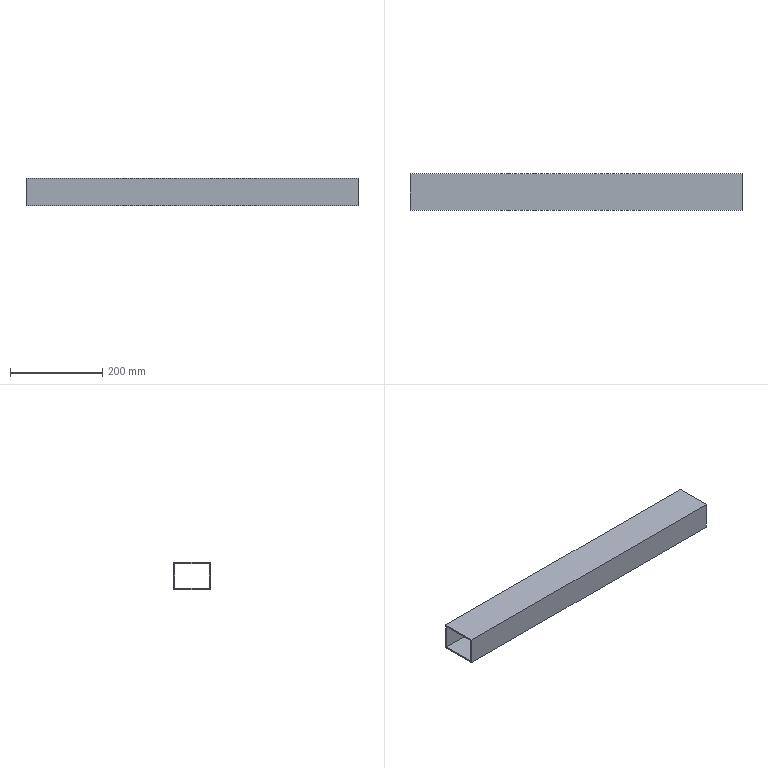Part | STEP file | Guide wheel mechanism revised.sldasm-Part-147 | 1 solid | 10 faces | box 720 x 80 x 60 mm | volume 578880 mm3 | plane 10
STEP:
#1=CARTESIAN_POINT('',(360.,1970.,200.));
#2=VERTEX_POINT('',#1);
#3=CARTESIAN_POINT('',(360.,1970.,260.));
#4=VERTEX_POINT('',#3);
#5=CARTESIAN_POINT('',(360.,1970.,260.));
#6=DIRECTION('',(0.,0.,1.));
#7=VECTOR('',#6,1000.);
#8=LINE('',#5,#7);
#9=EDGE_CURVE('',#2,#4,#8,.T.);
#10=ORIENTED_EDGE('',*,*,#9,.F.);
#11=CARTESIAN_POINT('',(-360.,1970.,200.));
#12=VERTEX_POINT('',#11);
#13=CARTESIAN_POINT('',(460.,1970.,200.));
#14=DIRECTION('',(-1.,0.,0.));
#15=VECTOR('',#14,1000.);
#16=LINE('',#13,#15);
#17=EDGE_CURVE('',#2,#12,#16,.T.);
#18=ORIENTED_EDGE('',*,*,#17,.T.);
#19=CARTESIAN_POINT('',(-360.,1970.,260.));
#20=VERTEX_POINT('',#19);
#21=CARTESIAN_POINT('',(-360.,1970.,260.));
#22=DIRECTION('',(0.,0.,1.));
#23=VECTOR('',#22,1000.);
#24=LINE('',#21,#23);
#25=EDGE_CURVE('',#12,#20,#24,.T.);
#26=ORIENTED_EDGE('',*,*,#25,.T.);
#27=CARTESIAN_POINT('',(460.,1970.,260.));
#28=DIRECTION('',(-1.,0.,0.));
#29=VECTOR('',#28,1000.);
#30=LINE('',#27,#29);
#31=EDGE_CURVE('',#4,#20,#30,.T.);
#32=ORIENTED_EDGE('',*,*,#31,.F.);
#33=EDGE_LOOP('',(#10,#18,#26,#32));
#34=FACE_OUTER_BOUND('',#33,.T.);
#35=CARTESIAN_POINT('',(460.,1970.,260.));
#36=DIRECTION('',(0.,-1.,0.));
#37=DIRECTION('',(0.,0.,-1.));
#38=AXIS2_PLACEMENT_3D('',#35,#36,#37);
#39=PLANE('',#38);
#40=ADVANCED_FACE('',(#34),#39,.F.);
#41=CARTESIAN_POINT('',(360.,1890.,200.));
#42=VERTEX_POINT('',#41);
#43=CARTESIAN_POINT('',(360.,1970.,200.));
#44=DIRECTION('',(0.,1.,0.));
#45=VECTOR('',#44,1000.);
#46=LINE('',#43,#45);
#47=EDGE_CURVE('',#42,#2,#46,.T.);
#48=ORIENTED_EDGE('',*,*,#47,.F.);
#49=CARTESIAN_POINT('',(-360.,1890.,200.));
#50=VERTEX_POINT('',#49);
#51=CARTESIAN_POINT('',(460.,1890.,200.));
#52=DIRECTION('',(-1.,0.,0.));
#53=VECTOR('',#52,1000.);
#54=LINE('',#51,#53);
#55=EDGE_CURVE('',#42,#50,#54,.T.);
#56=ORIENTED_EDGE('',*,*,#55,.T.);
#57=CARTESIAN_POINT('',(-360.,1970.,200.));
#58=DIRECTION('',(0.,1.,0.));
#59=VECTOR('',#58,1000.);
#60=LINE('',#57,#59);
#61=EDGE_CURVE('',#50,#12,#60,.T.);
#62=ORIENTED_EDGE('',*,*,#61,.T.);
#63=ORIENTED_EDGE('',*,*,#17,.F.);
#64=EDGE_LOOP('',(#48,#56,#62,#63));
#65=FACE_OUTER_BOUND('',#64,.T.);
#66=CARTESIAN_POINT('',(460.,1970.,200.));
#67=DIRECTION('',(0.,0.,1.));
#68=DIRECTION('',(1.,0.,0.));
#69=AXIS2_PLACEMENT_3D('',#66,#67,#68);
#70=PLANE('',#69);
#71=ADVANCED_FACE('',(#65),#70,.F.);
#72=CARTESIAN_POINT('',(360.,1890.,260.));
#73=VERTEX_POINT('',#72);
#74=CARTESIAN_POINT('',(360.,1890.,260.));
#75=DIRECTION('',(0.,0.,-1.));
#76=VECTOR('',#75,1000.);
#77=LINE('',#74,#76);
#78=EDGE_CURVE('',#73,#42,#77,.T.);
#79=ORIENTED_EDGE('',*,*,#78,.F.);
#80=CARTESIAN_POINT('',(-360.,1890.,260.));
#81=VERTEX_POINT('',#80);
#82=CARTESIAN_POINT('',(460.,1890.,260.));
#83=DIRECTION('',(-1.,0.,0.));
#84=VECTOR('',#83,1000.);
#85=LINE('',#82,#84);
#86=EDGE_CURVE('',#73,#81,#85,.T.);
#87=ORIENTED_EDGE('',*,*,#86,.T.);
#88=CARTESIAN_POINT('',(-360.,1890.,260.));
#89=DIRECTION('',(0.,0.,-1.));
#90=VECTOR('',#89,1000.);
#91=LINE('',#88,#90);
#92=EDGE_CURVE('',#81,#50,#91,.T.);
#93=ORIENTED_EDGE('',*,*,#92,.T.);
#94=ORIENTED_EDGE('',*,*,#55,.F.);
#95=EDGE_LOOP('',(#79,#87,#93,#94));
#96=FACE_OUTER_BOUND('',#95,.T.);
#97=CARTESIAN_POINT('',(460.,1890.,260.));
#98=DIRECTION('',(0.,1.,0.));
#99=DIRECTION('',(0.,0.,1.));
#100=AXIS2_PLACEMENT_3D('',#97,#98,#99);
#101=PLANE('',#100);
#102=ADVANCED_FACE('',(#96),#101,.F.);
#103=CARTESIAN_POINT('',(360.,1970.,260.));
#104=DIRECTION('',(0.,-1.,0.));
#105=VECTOR('',#104,1000.);
#106=LINE('',#103,#105);
#107=EDGE_CURVE('',#4,#73,#106,.T.);
#108=ORIENTED_EDGE('',*,*,#107,.F.);
#109=ORIENTED_EDGE('',*,*,#31,.T.);
#110=CARTESIAN_POINT('',(-360.,1970.,260.));
#111=DIRECTION('',(0.,-1.,0.));
#112=VECTOR('',#111,1000.);
#113=LINE('',#110,#112);
#114=EDGE_CURVE('',#20,#81,#113,.T.);
#115=ORIENTED_EDGE('',*,*,#114,.T.);
#116=ORIENTED_EDGE('',*,*,#86,.F.);
#117=EDGE_LOOP('',(#108,#109,#115,#116));
#118=FACE_OUTER_BOUND('',#117,.T.);
#119=CARTESIAN_POINT('',(460.,1970.,260.));
#120=DIRECTION('',(0.,0.,-1.));
#121=DIRECTION('',(0.,1.,0.));
#122=AXIS2_PLACEMENT_3D('',#119,#120,#121);
#123=PLANE('',#122);
#124=ADVANCED_FACE('',(#118),#123,.F.);
#125=ORIENTED_EDGE('',*,*,#114,.F.);
#126=ORIENTED_EDGE('',*,*,#25,.F.);
#127=ORIENTED_EDGE('',*,*,#61,.F.);
#128=ORIENTED_EDGE('',*,*,#92,.F.);
#129=EDGE_LOOP('',(#125,#126,#127,#128));
#130=FACE_OUTER_BOUND('',#129,.T.);
#131=CARTESIAN_POINT('',(-360.,1967.,257.));
#132=VERTEX_POINT('',#131);
#133=CARTESIAN_POINT('',(-360.,1893.,257.));
#134=VERTEX_POINT('',#133);
#135=CARTESIAN_POINT('',(-360.,1967.,257.));
#136=DIRECTION('',(0.,-1.,0.));
#137=VECTOR('',#136,1000.);
#138=LINE('',#135,#137);
#139=EDGE_CURVE('',#132,#134,#138,.T.);
#140=ORIENTED_EDGE('',*,*,#139,.T.);
#141=CARTESIAN_POINT('',(-360.,1893.,203.));
#142=VERTEX_POINT('',#141);
#143=CARTESIAN_POINT('',(-360.,1893.,257.));
#144=DIRECTION('',(0.,0.,-1.));
#145=VECTOR('',#144,1000.);
#146=LINE('',#143,#145);
#147=EDGE_CURVE('',#134,#142,#146,.T.);
#148=ORIENTED_EDGE('',*,*,#147,.T.);
#149=CARTESIAN_POINT('',(-360.,1967.,203.));
#150=VERTEX_POINT('',#149);
#151=CARTESIAN_POINT('',(-360.,1967.,203.));
#152=DIRECTION('',(0.,1.,0.));
#153=VECTOR('',#152,1000.);
#154=LINE('',#151,#153);
#155=EDGE_CURVE('',#142,#150,#154,.T.);
#156=ORIENTED_EDGE('',*,*,#155,.T.);
#157=CARTESIAN_POINT('',(-360.,1967.,257.));
#158=DIRECTION('',(0.,0.,1.));
#159=VECTOR('',#158,1000.);
#160=LINE('',#157,#159);
#161=EDGE_CURVE('',#150,#132,#160,.T.);
#162=ORIENTED_EDGE('',*,*,#161,.T.);
#163=EDGE_LOOP('',(#140,#148,#156,#162));
#164=FACE_BOUND('',#163,.T.);
#165=CARTESIAN_POINT('',(-360.,0.,0.));
#166=DIRECTION('',(1.,0.,0.));
#167=DIRECTION('',(0.,0.,-1.));
#168=AXIS2_PLACEMENT_3D('',#165,#166,#167);
#169=PLANE('',#168);
#170=ADVANCED_FACE('',(#130,#164),#169,.F.);
#171=CARTESIAN_POINT('',(360.,1967.,203.));
#172=VERTEX_POINT('',#171);
#173=CARTESIAN_POINT('',(460.,1967.,203.));
#174=DIRECTION('',(-1.,0.,0.));
#175=VECTOR('',#174,1000.);
#176=LINE('',#173,#175);
#177=EDGE_CURVE('',#172,#150,#176,.T.);
#178=ORIENTED_EDGE('',*,*,#177,.F.);
#179=CARTESIAN_POINT('',(360.,1967.,257.));
#180=VERTEX_POINT('',#179);
#181=CARTESIAN_POINT('',(360.,1967.,257.));
#182=DIRECTION('',(0.,0.,1.));
#183=VECTOR('',#182,1000.);
#184=LINE('',#181,#183);
#185=EDGE_CURVE('',#172,#180,#184,.T.);
#186=ORIENTED_EDGE('',*,*,#185,.T.);
#187=CARTESIAN_POINT('',(460.,1967.,257.));
#188=DIRECTION('',(-1.,0.,0.));
#189=VECTOR('',#188,1000.);
#190=LINE('',#187,#189);
#191=EDGE_CURVE('',#180,#132,#190,.T.);
#192=ORIENTED_EDGE('',*,*,#191,.T.);
#193=ORIENTED_EDGE('',*,*,#161,.F.);
#194=EDGE_LOOP('',(#178,#186,#192,#193));
#195=FACE_OUTER_BOUND('',#194,.T.);
#196=CARTESIAN_POINT('',(460.,1967.,257.));
#197=DIRECTION('',(0.,-1.,0.));
#198=DIRECTION('',(0.,0.,-1.));
#199=AXIS2_PLACEMENT_3D('',#196,#197,#198);
#200=PLANE('',#199);
#201=ADVANCED_FACE('',(#195),#200,.T.);
#202=CARTESIAN_POINT('',(360.,1893.,203.));
#203=VERTEX_POINT('',#202);
#204=CARTESIAN_POINT('',(460.,1893.,203.));
#205=DIRECTION('',(-1.,0.,0.));
#206=VECTOR('',#205,1000.);
#207=LINE('',#204,#206);
#208=EDGE_CURVE('',#203,#142,#207,.T.);
#209=ORIENTED_EDGE('',*,*,#208,.F.);
#210=CARTESIAN_POINT('',(360.,1967.,203.));
#211=DIRECTION('',(0.,1.,0.));
#212=VECTOR('',#211,1000.);
#213=LINE('',#210,#212);
#214=EDGE_CURVE('',#203,#172,#213,.T.);
#215=ORIENTED_EDGE('',*,*,#214,.T.);
#216=ORIENTED_EDGE('',*,*,#177,.T.);
#217=ORIENTED_EDGE('',*,*,#155,.F.);
#218=EDGE_LOOP('',(#209,#215,#216,#217));
#219=FACE_OUTER_BOUND('',#218,.T.);
#220=CARTESIAN_POINT('',(460.,1967.,203.));
#221=DIRECTION('',(0.,0.,1.));
#222=DIRECTION('',(1.,0.,0.));
#223=AXIS2_PLACEMENT_3D('',#220,#221,#222);
#224=PLANE('',#223);
#225=ADVANCED_FACE('',(#219),#224,.T.);
#226=CARTESIAN_POINT('',(360.,1893.,257.));
#227=VERTEX_POINT('',#226);
#228=CARTESIAN_POINT('',(460.,1893.,257.));
#229=DIRECTION('',(-1.,0.,0.));
#230=VECTOR('',#229,1000.);
#231=LINE('',#228,#230);
#232=EDGE_CURVE('',#227,#134,#231,.T.);
#233=ORIENTED_EDGE('',*,*,#232,.F.);
#234=CARTESIAN_POINT('',(360.,1893.,257.));
#235=DIRECTION('',(0.,0.,-1.));
#236=VECTOR('',#235,1000.);
#237=LINE('',#234,#236);
#238=EDGE_CURVE('',#227,#203,#237,.T.);
#239=ORIENTED_EDGE('',*,*,#238,.T.);
#240=ORIENTED_EDGE('',*,*,#208,.T.);
#241=ORIENTED_EDGE('',*,*,#147,.F.);
#242=EDGE_LOOP('',(#233,#239,#240,#241));
#243=FACE_OUTER_BOUND('',#242,.T.);
#244=CARTESIAN_POINT('',(460.,1893.,257.));
#245=DIRECTION('',(0.,1.,0.));
#246=DIRECTION('',(0.,0.,1.));
#247=AXIS2_PLACEMENT_3D('',#244,#245,#246);
#248=PLANE('',#247);
#249=ADVANCED_FACE('',(#243),#248,.T.);
#250=ORIENTED_EDGE('',*,*,#191,.F.);
#251=CARTESIAN_POINT('',(360.,1967.,257.));
#252=DIRECTION('',(0.,-1.,0.));
#253=VECTOR('',#252,1000.);
#254=LINE('',#251,#253);
#255=EDGE_CURVE('',#180,#227,#254,.T.);
#256=ORIENTED_EDGE('',*,*,#255,.T.);
#257=ORIENTED_EDGE('',*,*,#232,.T.);
#258=ORIENTED_EDGE('',*,*,#139,.F.);
#259=EDGE_LOOP('',(#250,#256,#257,#258));
#260=FACE_OUTER_BOUND('',#259,.T.);
#261=CARTESIAN_POINT('',(460.,1967.,257.));
#262=DIRECTION('',(0.,0.,-1.));
#263=DIRECTION('',(0.,1.,0.));
#264=AXIS2_PLACEMENT_3D('',#261,#262,#263);
#265=PLANE('',#264);
#266=ADVANCED_FACE('',(#260),#265,.T.);
#267=ORIENTED_EDGE('',*,*,#255,.F.);
#268=ORIENTED_EDGE('',*,*,#185,.F.);
#269=ORIENTED_EDGE('',*,*,#214,.F.);
#270=ORIENTED_EDGE('',*,*,#238,.F.);
#271=EDGE_LOOP('',(#267,#268,#269,#270));
#272=FACE_BOUND('',#271,.T.);
#273=ORIENTED_EDGE('',*,*,#9,.T.);
#274=ORIENTED_EDGE('',*,*,#107,.T.);
#275=ORIENTED_EDGE('',*,*,#78,.T.);
#276=ORIENTED_EDGE('',*,*,#47,.T.);
#277=EDGE_LOOP('',(#273,#274,#275,#276));
#278=FACE_OUTER_BOUND('',#277,.T.);
#279=CARTESIAN_POINT('',(360.,1970.,260.));
#280=DIRECTION('',(1.,0.,0.));
#281=DIRECTION('',(0.,0.,-1.));
#282=AXIS2_PLACEMENT_3D('',#279,#280,#281);
#283=PLANE('',#282);
#284=ADVANCED_FACE('',(#272,#278),#283,.T.);
#285=CLOSED_SHELL('',(#40,#71,#102,#124,#170,#201,#225,#249,#266,#284));
#286=MANIFOLD_SOLID_BREP('',#285);
#287=CARTESIAN_POINT('',(0.,0.,0.));
#288=DIRECTION('',(0.,0.,1.));
#289=DIRECTION('',(1.,0.,0.));
#290=AXIS2_PLACEMENT_3D('',#287,#288,#289);
#291=(LENGTH_UNIT()NAMED_UNIT(*)SI_UNIT(.MILLI.,.METRE.));
#292=UNCERTAINTY_MEASURE_WITH_UNIT(LENGTH_MEASURE(0.00001),#291,'','');
#293=(NAMED_UNIT(*)PLANE_ANGLE_UNIT()SI_UNIT($,.RADIAN.));
#294=(NAMED_UNIT(*)SI_UNIT($,.STERADIAN.)SOLID_ANGLE_UNIT());
#295=(GEOMETRIC_REPRESENTATION_CONTEXT(3)GLOBAL_UNCERTAINTY_ASSIGNED_CONTEXT((#292))GLOBAL_UNIT_ASSIGNED_CONTEXT((#291,#293,#294))REPRESENTATION_CONTEXT('',''));
#296=ADVANCED_BREP_SHAPE_REPRESENTATION('',(#286,#290),#295);